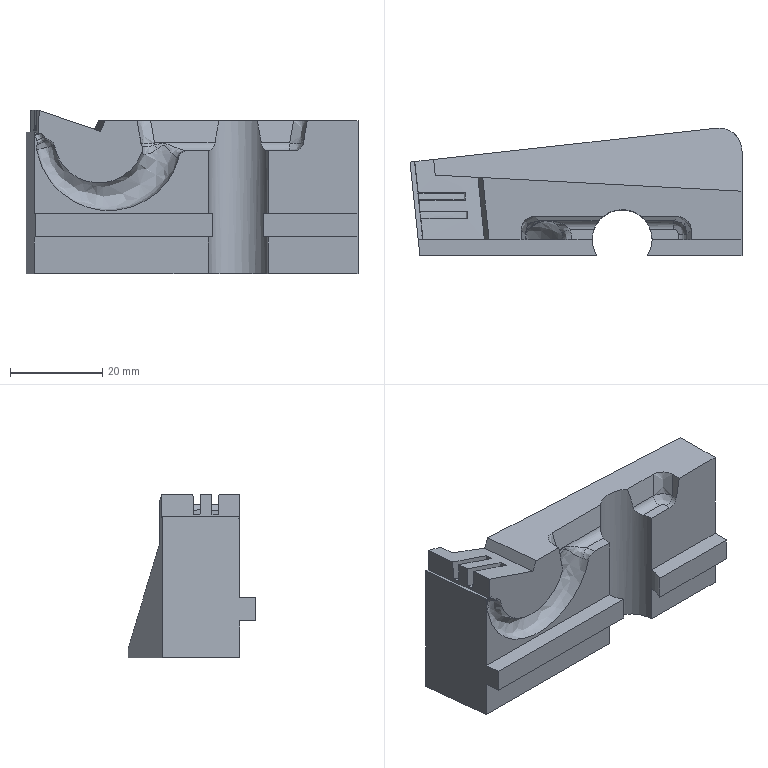Part | STEP file | P011002M007-000 | 1 solid | 55 faces | box 72.03 x 27.74 x 35.47 mm | volume 32998 mm3 | spline 26 | plane 22 | cylinder 4 | other 2 | cone 1 | commonest cylinder face diameters 4 x2 10 x1 13 x1